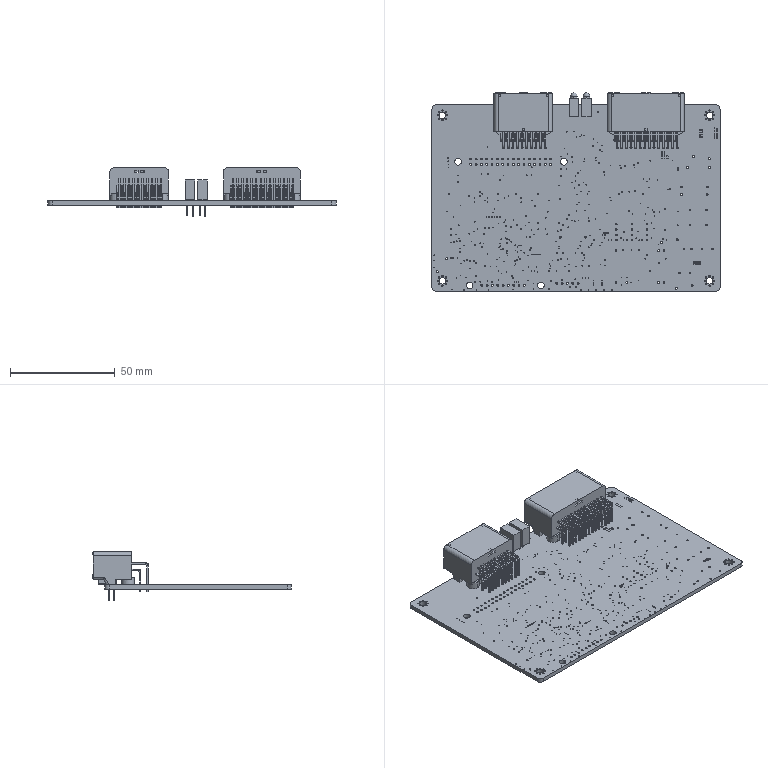Part | SolidWorks | 5 solids | 2557 faces | box 137.5 x 94.8 x 23.5 mm | volume 33178 mm3 | cylinder 1453 | plane 1102 | sphere 2 | commonest cylinder face diameters 0.305 x890 0.889 x112 1 x107 0.6 x64 0.381 x40 0.36 x28